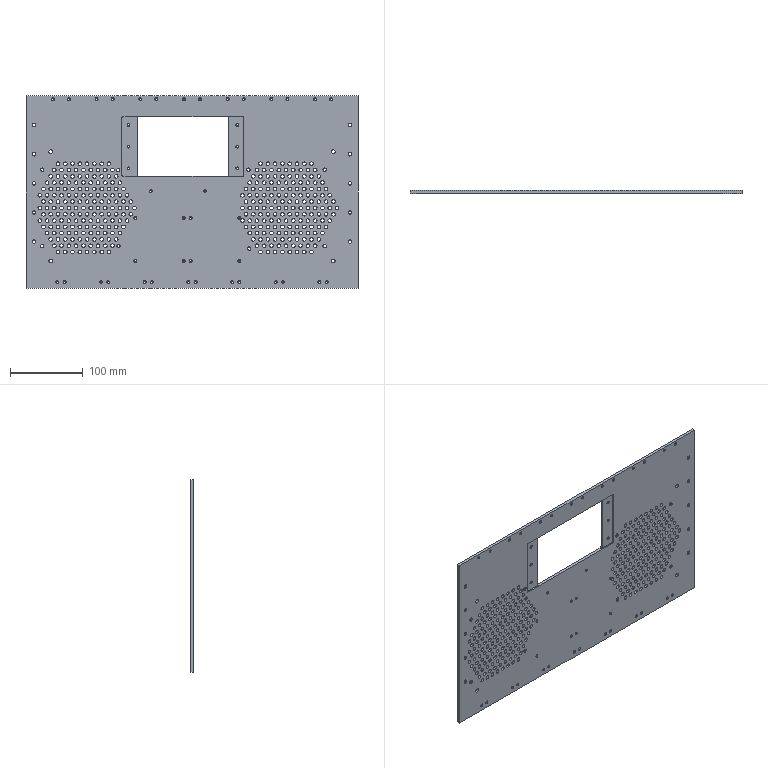Part | STEP file | Chassis front panel | 1 solid | 1014 faces | box 456 x 4 x 264.7 mm | volume 404809 mm3 | cylinder 406 | other 285 | plane 199 | cone 124 | commonest cylinder face diameters 5 x332 3.2 x44 4.3 x18 4 x8 5.1 x4